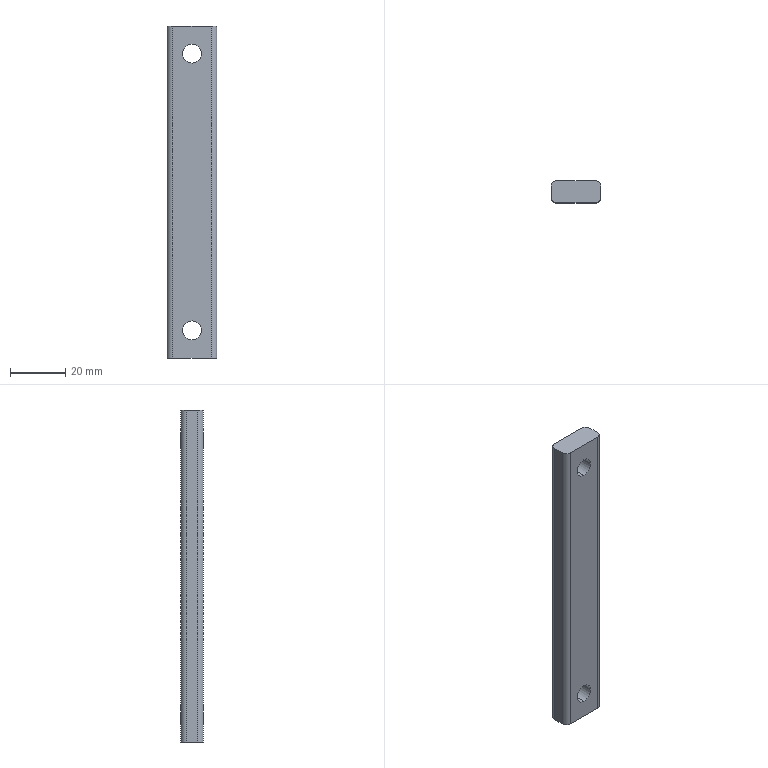Part | STEP file | Spring hanger hook | 1 solid | 14 faces | box 18 x 8 x 120 mm | volume 16287 mm3 | cylinder 8 | plane 6 | commonest cylinder face diameters 4 x4 6.8 x4
STEP:
#1=CARTESIAN_POINT('',(0.,0.,0.));
#2=DIRECTION('',(0.,0.,1.));
#3=DIRECTION('',(1.,0.,0.));
#4=AXIS2_PLACEMENT_3D('',#1,#2,#3);
#5=CARTESIAN_POINT('',(0.,4.,46.6));
#6=VERTEX_POINT('',#5);
#7=CARTESIAN_POINT('',(0.,-4.,46.6));
#8=VERTEX_POINT('',#7);
#9=CARTESIAN_POINT('',(0.,-4.,46.6));
#10=DIRECTION('',(0.,-1.,0.));
#11=VECTOR('',#10,1.);
#12=LINE('',#9,#11);
#13=CARTESIAN_POINT('',(0.,-4.,50.));
#14=DIRECTION('',(0.,-1.,0.));
#15=DIRECTION('',(0.,0.,-1.));
#16=AXIS2_PLACEMENT_3D('',#13,#14,#15);
#17=CYLINDRICAL_SURFACE('',#16,3.4);
#18=CARTESIAN_POINT('',(6.283,0.));
#19=DIRECTION('',(0.,1.));
#20=VECTOR('',#19,1.);
#21=LINE('',#18,#20);
#22=(GEOMETRIC_REPRESENTATION_CONTEXT(2)PARAMETRIC_REPRESENTATION_CONTEXT()REPRESENTATION_CONTEXT('',''));
#23=DEFINITIONAL_REPRESENTATION('',(#21),#22);
#24=PCURVE('',#17,#23);
#25=CARTESIAN_POINT('',(0.,-4.,50.));
#26=DIRECTION('',(0.,-1.,0.));
#27=DIRECTION('',(0.,0.,-1.));
#28=AXIS2_PLACEMENT_3D('',#25,#26,#27);
#29=CYLINDRICAL_SURFACE('',#28,3.4);
#30=CARTESIAN_POINT('',(0.,0.));
#31=DIRECTION('',(0.,1.));
#32=VECTOR('',#31,1.);
#33=LINE('',#30,#32);
#34=(GEOMETRIC_REPRESENTATION_CONTEXT(2)PARAMETRIC_REPRESENTATION_CONTEXT()REPRESENTATION_CONTEXT('',''));
#35=DEFINITIONAL_REPRESENTATION('',(#33),#34);
#36=PCURVE('',#29,#35);
#37=SURFACE_CURVE('',#12,(#24,#36),.PCURVE_S1.);
#38=EDGE_CURVE('',#6,#8,#37,.T.);
#39=ORIENTED_EDGE('',*,*,#38,.T.);
#40=CARTESIAN_POINT('',(0.,-4.,53.4));
#41=VERTEX_POINT('',#40);
#42=CARTESIAN_POINT('',(0.,-4.,50.));
#43=DIRECTION('',(0.,1.,0.));
#44=DIRECTION('',(0.,0.,-1.));
#45=AXIS2_PLACEMENT_3D('',#42,#43,#44);
#46=CIRCLE('',#45,3.4);
#47=CARTESIAN_POINT('',(6.283,0.));
#48=DIRECTION('',(-1.,0.));
#49=VECTOR('',#48,1.);
#50=LINE('',#47,#49);
#51=(GEOMETRIC_REPRESENTATION_CONTEXT(2)PARAMETRIC_REPRESENTATION_CONTEXT()REPRESENTATION_CONTEXT('',''));
#52=DEFINITIONAL_REPRESENTATION('',(#50),#51);
#53=PCURVE('',#17,#52);
#54=CARTESIAN_POINT('',(-9.,-4.,60.));
#55=DIRECTION('',(0.,1.,0.));
#56=DIRECTION('',(0.,0.,1.));
#57=AXIS2_PLACEMENT_3D('',#54,#55,#56);
#58=PLANE('',#57);
#59=CARTESIAN_POINT('',(-10.,9.));
#60=DIRECTION('',(-1.,0.));
#61=AXIS2_PLACEMENT_2D('',#59,#60);
#62=CIRCLE('',#61,3.4);
#63=(GEOMETRIC_REPRESENTATION_CONTEXT(2)PARAMETRIC_REPRESENTATION_CONTEXT()REPRESENTATION_CONTEXT('',''));
#64=DEFINITIONAL_REPRESENTATION('',(#62),#63);
#65=PCURVE('',#58,#64);
#66=SURFACE_CURVE('',#46,(#53,#65),.PCURVE_S1.);
#67=EDGE_CURVE('',#8,#41,#66,.T.);
#68=ORIENTED_EDGE('',*,*,#67,.T.);
#69=CARTESIAN_POINT('',(0.,4.,53.4));
#70=VERTEX_POINT('',#69);
#71=CARTESIAN_POINT('',(0.,-4.,53.4));
#72=DIRECTION('',(0.,-1.,0.));
#73=VECTOR('',#72,1.);
#74=LINE('',#71,#73);
#75=CARTESIAN_POINT('',(3.142,0.));
#76=DIRECTION('',(0.,1.));
#77=VECTOR('',#76,1.);
#78=LINE('',#75,#77);
#79=(GEOMETRIC_REPRESENTATION_CONTEXT(2)PARAMETRIC_REPRESENTATION_CONTEXT()REPRESENTATION_CONTEXT('',''));
#80=DEFINITIONAL_REPRESENTATION('',(#78),#79);
#81=PCURVE('',#17,#80);
#82=CARTESIAN_POINT('',(3.142,0.));
#83=DIRECTION('',(0.,1.));
#84=VECTOR('',#83,1.);
#85=LINE('',#82,#84);
#86=(GEOMETRIC_REPRESENTATION_CONTEXT(2)PARAMETRIC_REPRESENTATION_CONTEXT()REPRESENTATION_CONTEXT('',''));
#87=DEFINITIONAL_REPRESENTATION('',(#85),#86);
#88=PCURVE('',#29,#87);
#89=SURFACE_CURVE('',#74,(#81,#88),.PCURVE_S1.);
#90=EDGE_CURVE('',#70,#41,#89,.T.);
#91=ORIENTED_EDGE('',*,*,#90,.F.);
#92=CARTESIAN_POINT('',(0.,4.,50.));
#93=DIRECTION('',(0.,1.,0.));
#94=DIRECTION('',(0.,0.,-1.));
#95=AXIS2_PLACEMENT_3D('',#92,#93,#94);
#96=CIRCLE('',#95,3.4);
#97=CARTESIAN_POINT('',(6.283,-8.));
#98=DIRECTION('',(-1.,0.));
#99=VECTOR('',#98,1.);
#100=LINE('',#97,#99);
#101=(GEOMETRIC_REPRESENTATION_CONTEXT(2)PARAMETRIC_REPRESENTATION_CONTEXT()REPRESENTATION_CONTEXT('',''));
#102=DEFINITIONAL_REPRESENTATION('',(#100),#101);
#103=PCURVE('',#17,#102);
#104=CARTESIAN_POINT('',(-9.,4.,60.));
#105=DIRECTION('',(0.,-1.,0.));
#106=DIRECTION('',(0.,0.,-1.));
#107=AXIS2_PLACEMENT_3D('',#104,#105,#106);
#108=PLANE('',#107);
#109=CARTESIAN_POINT('',(13.4,9.));
#110=CARTESIAN_POINT('',(13.4,3.111));
#111=CARTESIAN_POINT('',(8.3,6.056));
#112=CARTESIAN_POINT('',(3.2,9.));
#113=CARTESIAN_POINT('',(8.3,11.944));
#114=CARTESIAN_POINT('',(13.4,14.889));
#115=CARTESIAN_POINT('',(13.4,9.));
#116=(BOUNDED_CURVE()B_SPLINE_CURVE(2,(#109,#110,#111,#112,#113,#114,#115),.UNSPECIFIED.,.T.,.F.)B_SPLINE_CURVE_WITH_KNOTS((1,2,2,2,2,1),(-2.094,0.,2.094,4.189,6.283,8.378),.UNSPECIFIED.)CURVE()GEOMETRIC_REPRESENTATION_ITEM()RATIONAL_B_SPLINE_CURVE((1.,0.5,1.,0.5,1.,0.5,1.))REPRESENTATION_ITEM(''));
#117=(GEOMETRIC_REPRESENTATION_CONTEXT(2)PARAMETRIC_REPRESENTATION_CONTEXT()REPRESENTATION_CONTEXT('',''));
#118=DEFINITIONAL_REPRESENTATION('',(#116),#117);
#119=PCURVE('',#108,#118);
#120=SURFACE_CURVE('',#96,(#103,#119),.PCURVE_S1.);
#121=EDGE_CURVE('',#6,#70,#120,.T.);
#122=ORIENTED_EDGE('',*,*,#121,.F.);
#123=EDGE_LOOP('',(#39,#68,#91,#122));
#124=FACE_BOUND('',#123,.F.);
#125=ADVANCED_FACE('',(#124),#17,.F.);
#126=CARTESIAN_POINT('',(0.,4.,-53.4));
#127=VERTEX_POINT('',#126);
#128=CARTESIAN_POINT('',(0.,-4.,-53.4));
#129=VERTEX_POINT('',#128);
#130=CARTESIAN_POINT('',(0.,-4.,-53.4));
#131=DIRECTION('',(0.,-1.,0.));
#132=VECTOR('',#131,1.);
#133=LINE('',#130,#132);
#134=CARTESIAN_POINT('',(0.,-4.,-50.));
#135=DIRECTION('',(0.,-1.,0.));
#136=DIRECTION('',(0.,0.,-1.));
#137=AXIS2_PLACEMENT_3D('',#134,#135,#136);
#138=CYLINDRICAL_SURFACE('',#137,3.4);
#139=CARTESIAN_POINT('',(6.283,0.));
#140=DIRECTION('',(0.,1.));
#141=VECTOR('',#140,1.);
#142=LINE('',#139,#141);
#143=(GEOMETRIC_REPRESENTATION_CONTEXT(2)PARAMETRIC_REPRESENTATION_CONTEXT()REPRESENTATION_CONTEXT('',''));
#144=DEFINITIONAL_REPRESENTATION('',(#142),#143);
#145=PCURVE('',#138,#144);
#146=CARTESIAN_POINT('',(0.,-4.,-50.));
#147=DIRECTION('',(0.,-1.,0.));
#148=DIRECTION('',(0.,0.,-1.));
#149=AXIS2_PLACEMENT_3D('',#146,#147,#148);
#150=CYLINDRICAL_SURFACE('',#149,3.4);
#151=CARTESIAN_POINT('',(0.,0.));
#152=DIRECTION('',(0.,1.));
#153=VECTOR('',#152,1.);
#154=LINE('',#151,#153);
#155=(GEOMETRIC_REPRESENTATION_CONTEXT(2)PARAMETRIC_REPRESENTATION_CONTEXT()REPRESENTATION_CONTEXT('',''));
#156=DEFINITIONAL_REPRESENTATION('',(#154),#155);
#157=PCURVE('',#150,#156);
#158=SURFACE_CURVE('',#133,(#145,#157),.PCURVE_S1.);
#159=EDGE_CURVE('',#127,#129,#158,.T.);
#160=ORIENTED_EDGE('',*,*,#159,.T.);
#161=CARTESIAN_POINT('',(0.,-4.,-46.6));
#162=VERTEX_POINT('',#161);
#163=CARTESIAN_POINT('',(0.,-4.,-50.));
#164=DIRECTION('',(0.,1.,0.));
#165=DIRECTION('',(0.,0.,-1.));
#166=AXIS2_PLACEMENT_3D('',#163,#164,#165);
#167=CIRCLE('',#166,3.4);
#168=CARTESIAN_POINT('',(6.283,0.));
#169=DIRECTION('',(-1.,0.));
#170=VECTOR('',#169,1.);
#171=LINE('',#168,#170);
#172=(GEOMETRIC_REPRESENTATION_CONTEXT(2)PARAMETRIC_REPRESENTATION_CONTEXT()REPRESENTATION_CONTEXT('',''));
#173=DEFINITIONAL_REPRESENTATION('',(#171),#172);
#174=PCURVE('',#138,#173);
#175=CARTESIAN_POINT('',(-110.,9.));
#176=DIRECTION('',(-1.,0.));
#177=AXIS2_PLACEMENT_2D('',#175,#176);
#178=CIRCLE('',#177,3.4);
#179=(GEOMETRIC_REPRESENTATION_CONTEXT(2)PARAMETRIC_REPRESENTATION_CONTEXT()REPRESENTATION_CONTEXT('',''));
#180=DEFINITIONAL_REPRESENTATION('',(#178),#179);
#181=PCURVE('',#58,#180);
#182=SURFACE_CURVE('',#167,(#174,#181),.PCURVE_S1.);
#183=EDGE_CURVE('',#129,#162,#182,.T.);
#184=ORIENTED_EDGE('',*,*,#183,.T.);
#185=CARTESIAN_POINT('',(0.,4.,-46.6));
#186=VERTEX_POINT('',#185);
#187=CARTESIAN_POINT('',(0.,-4.,-46.6));
#188=DIRECTION('',(0.,-1.,0.));
#189=VECTOR('',#188,1.);
#190=LINE('',#187,#189);
#191=CARTESIAN_POINT('',(3.142,0.));
#192=DIRECTION('',(0.,1.));
#193=VECTOR('',#192,1.);
#194=LINE('',#191,#193);
#195=(GEOMETRIC_REPRESENTATION_CONTEXT(2)PARAMETRIC_REPRESENTATION_CONTEXT()REPRESENTATION_CONTEXT('',''));
#196=DEFINITIONAL_REPRESENTATION('',(#194),#195);
#197=PCURVE('',#138,#196);
#198=CARTESIAN_POINT('',(3.142,0.));
#199=DIRECTION('',(0.,1.));
#200=VECTOR('',#199,1.);
#201=LINE('',#198,#200);
#202=(GEOMETRIC_REPRESENTATION_CONTEXT(2)PARAMETRIC_REPRESENTATION_CONTEXT()REPRESENTATION_CONTEXT('',''));
#203=DEFINITIONAL_REPRESENTATION('',(#201),#202);
#204=PCURVE('',#150,#203);
#205=SURFACE_CURVE('',#190,(#197,#204),.PCURVE_S1.);
#206=EDGE_CURVE('',#186,#162,#205,.T.);
#207=ORIENTED_EDGE('',*,*,#206,.F.);
#208=CARTESIAN_POINT('',(0.,4.,-50.));
#209=DIRECTION('',(0.,1.,0.));
#210=DIRECTION('',(0.,0.,-1.));
#211=AXIS2_PLACEMENT_3D('',#208,#209,#210);
#212=CIRCLE('',#211,3.4);
#213=CARTESIAN_POINT('',(6.283,-8.));
#214=DIRECTION('',(-1.,0.));
#215=VECTOR('',#214,1.);
#216=LINE('',#213,#215);
#217=(GEOMETRIC_REPRESENTATION_CONTEXT(2)PARAMETRIC_REPRESENTATION_CONTEXT()REPRESENTATION_CONTEXT('',''));
#218=DEFINITIONAL_REPRESENTATION('',(#216),#217);
#219=PCURVE('',#138,#218);
#220=CARTESIAN_POINT('',(113.4,9.));
#221=CARTESIAN_POINT('',(113.4,3.111));
#222=CARTESIAN_POINT('',(108.3,6.056));
#223=CARTESIAN_POINT('',(103.2,9.));
#224=CARTESIAN_POINT('',(108.3,11.944));
#225=CARTESIAN_POINT('',(113.4,14.889));
#226=CARTESIAN_POINT('',(113.4,9.));
#227=(BOUNDED_CURVE()B_SPLINE_CURVE(2,(#220,#221,#222,#223,#224,#225,#226),.UNSPECIFIED.,.T.,.F.)B_SPLINE_CURVE_WITH_KNOTS((1,2,2,2,2,1),(-2.094,0.,2.094,4.189,6.283,8.378),.UNSPECIFIED.)CURVE()GEOMETRIC_REPRESENTATION_ITEM()RATIONAL_B_SPLINE_CURVE((1.,0.5,1.,0.5,1.,0.5,1.))REPRESENTATION_ITEM(''));
#228=(GEOMETRIC_REPRESENTATION_CONTEXT(2)PARAMETRIC_REPRESENTATION_CONTEXT()REPRESENTATION_CONTEXT('',''));
#229=DEFINITIONAL_REPRESENTATION('',(#227),#228);
#230=PCURVE('',#108,#229);
#231=SURFACE_CURVE('',#212,(#219,#230),.PCURVE_S1.);
#232=EDGE_CURVE('',#127,#186,#231,.T.);
#233=ORIENTED_EDGE('',*,*,#232,.F.);
#234=EDGE_LOOP('',(#160,#184,#207,#233));
#235=FACE_BOUND('',#234,.F.);
#236=ADVANCED_FACE('',(#235),#138,.F.);
#237=CARTESIAN_POINT('',(-7.,4.,60.));
#238=VERTEX_POINT('',#237);
#239=CARTESIAN_POINT('',(-7.,4.,-60.));
#240=VERTEX_POINT('',#239);
#241=CARTESIAN_POINT('',(-7.,4.,60.));
#242=DIRECTION('',(0.,0.,-1.));
#243=VECTOR('',#242,1.);
#244=LINE('',#241,#243);
#245=CARTESIAN_POINT('',(0.,2.));
#246=DIRECTION('',(1.,0.));
#247=VECTOR('',#246,1.);
#248=LINE('',#245,#247);
#249=(GEOMETRIC_REPRESENTATION_CONTEXT(2)PARAMETRIC_REPRESENTATION_CONTEXT()REPRESENTATION_CONTEXT('',''));
#250=DEFINITIONAL_REPRESENTATION('',(#248),#249);
#251=PCURVE('',#108,#250);
#252=CARTESIAN_POINT('',(-7.,2.,60.));
#253=DIRECTION('',(0.,0.,-1.));
#254=DIRECTION('',(-1.,0.,0.));
#255=AXIS2_PLACEMENT_3D('',#252,#253,#254);
#256=CYLINDRICAL_SURFACE('',#255,2.);
#257=CARTESIAN_POINT('',(1.571,0.));
#258=DIRECTION('',(0.,1.));
#259=VECTOR('',#258,1.);
#260=LINE('',#257,#259);
#261=(GEOMETRIC_REPRESENTATION_CONTEXT(2)PARAMETRIC_REPRESENTATION_CONTEXT()REPRESENTATION_CONTEXT('',''));
#262=DEFINITIONAL_REPRESENTATION('',(#260),#261);
#263=PCURVE('',#256,#262);
#264=SURFACE_CURVE('',#244,(#251,#263),.PCURVE_S1.);
#265=EDGE_CURVE('',#238,#240,#264,.T.);
#266=ORIENTED_EDGE('',*,*,#265,.F.);
#267=CARTESIAN_POINT('',(7.,4.,60.));
#268=VERTEX_POINT('',#267);
#269=CARTESIAN_POINT('',(-9.,4.,60.));
#270=DIRECTION('',(-1.,0.,0.));
#271=VECTOR('',#270,1.);
#272=LINE('',#269,#271);
#273=CARTESIAN_POINT('',(0.,0.));
#274=DIRECTION('',(0.,-1.));
#275=VECTOR('',#274,1.);
#276=LINE('',#273,#275);
#277=(GEOMETRIC_REPRESENTATION_CONTEXT(2)PARAMETRIC_REPRESENTATION_CONTEXT()REPRESENTATION_CONTEXT('',''));
#278=DEFINITIONAL_REPRESENTATION('',(#276),#277);
#279=PCURVE('',#108,#278);
#280=CARTESIAN_POINT('',(9.,-4.,60.));
#281=DIRECTION('',(0.,0.,1.));
#282=DIRECTION('',(1.,0.,0.));
#283=AXIS2_PLACEMENT_3D('',#280,#281,#282);
#284=PLANE('',#283);
#285=CARTESIAN_POINT('',(-18.,8.));
#286=DIRECTION('',(-1.,0.));
#287=VECTOR('',#286,1.);
#288=LINE('',#285,#287);
#289=(GEOMETRIC_REPRESENTATION_CONTEXT(2)PARAMETRIC_REPRESENTATION_CONTEXT()REPRESENTATION_CONTEXT('',''));
#290=DEFINITIONAL_REPRESENTATION('',(#288),#289);
#291=PCURVE('',#284,#290);
#292=SURFACE_CURVE('',#272,(#279,#291),.PCURVE_S1.);
#293=EDGE_CURVE('',#268,#238,#292,.T.);
#294=ORIENTED_EDGE('',*,*,#293,.F.);
#295=CARTESIAN_POINT('',(7.,4.,-60.));
#296=VERTEX_POINT('',#295);
#297=CARTESIAN_POINT('',(7.,4.,60.));
#298=DIRECTION('',(0.,0.,1.));
#299=VECTOR('',#298,1.);
#300=LINE('',#297,#299);
#301=CARTESIAN_POINT('',(0.,16.));
#302=DIRECTION('',(-1.,0.));
#303=VECTOR('',#302,1.);
#304=LINE('',#301,#303);
#305=(GEOMETRIC_REPRESENTATION_CONTEXT(2)PARAMETRIC_REPRESENTATION_CONTEXT()REPRESENTATION_CONTEXT('',''));
#306=DEFINITIONAL_REPRESENTATION('',(#304),#305);
#307=PCURVE('',#108,#306);
#308=CARTESIAN_POINT('',(7.,2.,60.));
#309=DIRECTION('',(0.,0.,-1.));
#310=DIRECTION('',(-1.,0.,0.));
#311=AXIS2_PLACEMENT_3D('',#308,#309,#310);
#312=CYLINDRICAL_SURFACE('',#311,2.);
#313=CARTESIAN_POINT('',(1.571,0.));
#314=DIRECTION('',(0.,-1.));
#315=VECTOR('',#314,1.);
#316=LINE('',#313,#315);
#317=(GEOMETRIC_REPRESENTATION_CONTEXT(2)PARAMETRIC_REPRESENTATION_CONTEXT()REPRESENTATION_CONTEXT('',''));
#318=DEFINITIONAL_REPRESENTATION('',(#316),#317);
#319=PCURVE('',#312,#318);
#320=SURFACE_CURVE('',#300,(#307,#319),.PCURVE_S1.);
#321=EDGE_CURVE('',#296,#268,#320,.T.);
#322=ORIENTED_EDGE('',*,*,#321,.F.);
#323=CARTESIAN_POINT('',(-9.,4.,-60.));
#324=DIRECTION('',(1.,0.,0.));
#325=VECTOR('',#324,1.);
#326=LINE('',#323,#325);
#327=CARTESIAN_POINT('',(120.,0.));
#328=DIRECTION('',(0.,1.));
#329=VECTOR('',#328,1.);
#330=LINE('',#327,#329);
#331=(GEOMETRIC_REPRESENTATION_CONTEXT(2)PARAMETRIC_REPRESENTATION_CONTEXT()REPRESENTATION_CONTEXT('',''));
#332=DEFINITIONAL_REPRESENTATION('',(#330),#331);
#333=PCURVE('',#108,#332);
#334=CARTESIAN_POINT('',(9.,-4.,-60.));
#335=DIRECTION('',(0.,0.,1.));
#336=DIRECTION('',(1.,0.,0.));
#337=AXIS2_PLACEMENT_3D('',#334,#335,#336);
#338=PLANE('',#337);
#339=CARTESIAN_POINT('',(-18.,8.));
#340=DIRECTION('',(1.,0.));
#341=VECTOR('',#340,1.);
#342=LINE('',#339,#341);
#343=(GEOMETRIC_REPRESENTATION_CONTEXT(2)PARAMETRIC_REPRESENTATION_CONTEXT()REPRESENTATION_CONTEXT('',''));
#344=DEFINITIONAL_REPRESENTATION('',(#342),#343);
#345=PCURVE('',#338,#344);
#346=SURFACE_CURVE('',#326,(#333,#345),.PCURVE_S1.);
#347=EDGE_CURVE('',#240,#296,#346,.T.);
#348=ORIENTED_EDGE('',*,*,#347,.F.);
#349=EDGE_LOOP('',(#266,#294,#322,#348));
#350=FACE_BOUND('',#349,.T.);
#351=ORIENTED_EDGE('',*,*,#121,.F.);
#352=CARTESIAN_POINT('',(0.,4.,50.));
#353=DIRECTION('',(0.,1.,0.));
#354=DIRECTION('',(0.,0.,-1.));
#355=AXIS2_PLACEMENT_3D('',#352,#353,#354);
#356=CIRCLE('',#355,3.4);
#357=CARTESIAN_POINT('',(13.4,9.));
#358=CARTESIAN_POINT('',(13.4,3.111));
#359=CARTESIAN_POINT('',(8.3,6.056));
#360=CARTESIAN_POINT('',(3.2,9.));
#361=CARTESIAN_POINT('',(8.3,11.944));
#362=CARTESIAN_POINT('',(13.4,14.889));
#363=CARTESIAN_POINT('',(13.4,9.));
#364=(BOUNDED_CURVE()B_SPLINE_CURVE(2,(#357,#358,#359,#360,#361,#362,#363),.UNSPECIFIED.,.T.,.F.)B_SPLINE_CURVE_WITH_KNOTS((1,2,2,2,2,1),(-2.094,0.,2.094,4.189,6.283,8.378),.UNSPECIFIED.)CURVE()GEOMETRIC_REPRESENTATION_ITEM()RATIONAL_B_SPLINE_CURVE((1.,0.5,1.,0.5,1.,0.5,1.))REPRESENTATION_ITEM(''));
#365=(GEOMETRIC_REPRESENTATION_CONTEXT(2)PARAMETRIC_REPRESENTATION_CONTEXT()REPRESENTATION_CONTEXT('',''));
#366=DEFINITIONAL_REPRESENTATION('',(#364),#365);
#367=PCURVE('',#108,#366);
#368=CARTESIAN_POINT('',(6.283,-8.));
#369=DIRECTION('',(-1.,0.));
#370=VECTOR('',#369,1.);
#371=LINE('',#368,#370);
#372=(GEOMETRIC_REPRESENTATION_CONTEXT(2)PARAMETRIC_REPRESENTATION_CONTEXT()REPRESENTATION_CONTEXT('',''));
#373=DEFINITIONAL_REPRESENTATION('',(#371),#372);
#374=PCURVE('',#29,#373);
#375=SURFACE_CURVE('',#356,(#367,#374),.PCURVE_S1.);
#376=EDGE_CURVE('',#70,#6,#375,.T.);
#377=ORIENTED_EDGE('',*,*,#376,.F.);
#378=EDGE_LOOP('',(#351,#377));
#379=FACE_BOUND('',#378,.T.);
#380=ORIENTED_EDGE('',*,*,#232,.F.);
#381=CARTESIAN_POINT('',(0.,4.,-50.));
#382=DIRECTION('',(0.,1.,0.));
#383=DIRECTION('',(0.,0.,-1.));
#384=AXIS2_PLACEMENT_3D('',#381,#382,#383);
#385=CIRCLE('',#384,3.4);
#386=CARTESIAN_POINT('',(113.4,9.));
#387=CARTESIAN_POINT('',(113.4,3.111));
#388=CARTESIAN_POINT('',(108.3,6.056));
#389=CARTESIAN_POINT('',(103.2,9.));
#390=CARTESIAN_POINT('',(108.3,11.944));
#391=CARTESIAN_POINT('',(113.4,14.889));
#392=CARTESIAN_POINT('',(113.4,9.));
#393=(BOUNDED_CURVE()B_SPLINE_CURVE(2,(#386,#387,#388,#389,#390,#391,#392),.UNSPECIFIED.,.T.,.F.)B_SPLINE_CURVE_WITH_KNOTS((1,2,2,2,2,1),(-2.094,0.,2.094,4.189,6.283,8.378),.UNSPECIFIED.)CURVE()GEOMETRIC_REPRESENTATION_ITEM()RATIONAL_B_SPLINE_CURVE((1.,0.5,1.,0.5,1.,0.5,1.))REPRESENTATION_ITEM(''));
#394=(GEOMETRIC_REPRESENTATION_CONTEXT(2)PARAMETRIC_REPRESENTATION_CONTEXT()REPRESENTATION_CONTEXT('',''));
#395=DEFINITIONAL_REPRESENTATION('',(#393),#394);
#396=PCURVE('',#108,#395);
#397=CARTESIAN_POINT('',(6.283,-8.));
#398=DIRECTION('',(-1.,0.));
#399=VECTOR('',#398,1.);
#400=LINE('',#397,#399);
#401=(GEOMETRIC_REPRESENTATION_CONTEXT(2)PARAMETRIC_REPRESENTATION_CONTEXT()REPRESENTATION_CONTEXT('',''));
#402=DEFINITIONAL_REPRESENTATION('',(#400),#401);
#403=PCURVE('',#150,#402);
#404=SURFACE_CURVE('',#385,(#396,#403),.PCURVE_S1.);
#405=EDGE_CURVE('',#186,#127,#404,.T.);
#406=ORIENTED_EDGE('',*,*,#405,.F.);
#407=EDGE_LOOP('',(#380,#406));
#408=FACE_BOUND('',#407,.T.);
#409=ADVANCED_FACE('',(#350,#379,#408),#108,.F.);
#410=CARTESIAN_POINT('',(-9.,-2.,-60.));
#411=VERTEX_POINT('',#410);
#412=CARTESIAN_POINT('',(-7.,-4.,-60.));
#413=VERTEX_POINT('',#412);
#414=CARTESIAN_POINT('',(-7.,-2.,-60.));
#415=DIRECTION('',(0.,0.,1.));
#416=DIRECTION('',(-1.,0.,0.));
#417=AXIS2_PLACEMENT_3D('',#414,#415,#416);
#418=CIRCLE('',#417,2.);
#419=CARTESIAN_POINT('',(-16.,2.));
#420=DIRECTION('',(-1.,0.));
#421=AXIS2_PLACEMENT_2D('',#419,#420);
#422=CIRCLE('',#421,2.);
#423=(GEOMETRIC_REPRESENTATION_CONTEXT(2)PARAMETRIC_REPRESENTATION_CONTEXT()REPRESENTATION_CONTEXT('',''));
#424=DEFINITIONAL_REPRESENTATION('',(#422),#423);
#425=PCURVE('',#338,#424);
#426=CARTESIAN_POINT('',(-7.,-2.,60.));
#427=DIRECTION('',(0.,0.,-1.));
#428=DIRECTION('',(-1.,0.,0.));
#429=AXIS2_PLACEMENT_3D('',#426,#427,#428);
#430=CYLINDRICAL_SURFACE('',#429,2.);
#431=CARTESIAN_POINT('',(6.283,120.));
#432=DIRECTION('',(-1.,0.));
#433=VECTOR('',#432,1.);
#434=LINE('',#431,#433);
#435=(GEOMETRIC_REPRESENTATION_CONTEXT(2)PARAMETRIC_REPRESENTATION_CONTEXT()REPRESENTATION_CONTEXT('',''));
#436=DEFINITIONAL_REPRESENTATION('',(#434),#435);
#437=PCURVE('',#430,#436);
#438=SURFACE_CURVE('',#418,(#425,#437),.PCURVE_S1.);
#439=EDGE_CURVE('',#411,#413,#438,.T.);
#440=ORIENTED_EDGE('',*,*,#439,.F.);
#441=CARTESIAN_POINT('',(-9.,2.,-60.));
#442=VERTEX_POINT('',#441);
#443=CARTESIAN_POINT('',(-9.,-4.,-60.));
#444=DIRECTION('',(0.,-1.,0.));
#445=VECTOR('',#444,1.);
#446=LINE('',#443,#445);
#447=CARTESIAN_POINT('',(-18.,0.));
#448=DIRECTION('',(0.,-1.));
#449=VECTOR('',#448,1.);
#450=LINE('',#447,#449);
#451=(GEOMETRIC_REPRESENTATION_CONTEXT(2)PARAMETRIC_REPRESENTATION_CONTEXT()REPRESENTATION_CONTEXT('',''));
#452=DEFINITIONAL_REPRESENTATION('',(#450),#451);
#453=PCURVE('',#338,#452);
#454=CARTESIAN_POINT('',(-9.,4.,60.));
#455=DIRECTION('',(1.,0.,0.));
#456=DIRECTION('',(0.,1.,0.));
#457=AXIS2_PLACEMENT_3D('',#454,#455,#456);
#458=PLANE('',#457);
#459=CARTESIAN_POINT('',(-8.,-120.));
#460=DIRECTION('',(-1.,0.));
#461=VECTOR('',#460,1.);
#462=LINE('',#459,#461);
#463=(GEOMETRIC_REPRESENTATION_CONTEXT(2)PARAMETRIC_REPRESENTATION_CONTEXT()REPRESENTATION_CONTEXT('',''));
#464=DEFINITIONAL_REPRESENTATION('',(#462),#463);
#465=PCURVE('',#458,#464);
#466=SURFACE_CURVE('',#446,(#453,#465),.PCURVE_S1.);
#467=EDGE_CURVE('',#442,#411,#466,.T.);
#468=ORIENTED_EDGE('',*,*,#467,.F.);
#469=CARTESIAN_POINT('',(-7.,2.,-60.));
#470=DIRECTION('',(0.,0.,1.));
#471=DIRECTION('',(-1.,0.,0.));
#472=AXIS2_PLACEMENT_3D('',#469,#470,#471);
#473=CIRCLE('',#472,2.);
#474=CARTESIAN_POINT('',(-16.,6.));
#475=DIRECTION('',(-1.,0.));
#476=AXIS2_PLACEMENT_2D('',#474,#475);
#477=CIRCLE('',#476,2.);
#478=(GEOMETRIC_REPRESENTATION_CONTEXT(2)PARAMETRIC_REPRESENTATION_CONTEXT()REPRESENTATION_CONTEXT('',''));
#479=DEFINITIONAL_REPRESENTATION('',(#477),#478);
#480=PCURVE('',#338,#479);
#481=CARTESIAN_POINT('',(6.283,120.));
#482=DIRECTION('',(-1.,0.));
#483=VECTOR('',#482,1.);
#484=LINE('',#481,#483);
#485=(GEOMETRIC_REPRESENTATION_CONTEXT(2)PARAMETRIC_REPRESENTATION_CONTEXT()REPRESENTATION_CONTEXT('',''));
#486=DEFINITIONAL_REPRESENTATION('',(#484),#485);
#487=PCURVE('',#256,#486);
#488=SURFACE_CURVE('',#473,(#480,#487),.PCURVE_S1.);
#489=EDGE_CURVE('',#240,#442,#488,.T.);
#490=ORIENTED_EDGE('',*,*,#489,.F.);
#491=ORIENTED_EDGE('',*,*,#347,.T.);
#492=CARTESIAN_POINT('',(9.,2.,-60.));
#493=VERTEX_POINT('',#492);
#494=CARTESIAN_POINT('',(7.,2.,-60.));
#495=DIRECTION('',(0.,0.,1.));
#496=DIRECTION('',(-1.,0.,0.));
#497=AXIS2_PLACEMENT_3D('',#494,#495,#496);
#498=CIRCLE('',#497,2.);
#499=CARTESIAN_POINT('',(-2.,6.));
#500=DIRECTION('',(-1.,0.));
#501=AXIS2_PLACEMENT_2D('',#499,#500);
#502=CIRCLE('',#501,2.);
#503=(GEOMETRIC_REPRESENTATION_CONTEXT(2)PARAMETRIC_REPRESENTATION_CONTEXT()REPRESENTATION_CONTEXT('',''));
#504=DEFINITIONAL_REPRESENTATION('',(#502),#503);
#505=PCURVE('',#338,#504);
#506=CARTESIAN_POINT('',(6.283,120.));
#507=DIRECTION('',(-1.,0.));
#508=VECTOR('',#507,1.);
#509=LINE('',#506,#508);
#510=(GEOMETRIC_REPRESENTATION_CONTEXT(2)PARAMETRIC_REPRESENTATION_CONTEXT()REPRESENTATION_CONTEXT('',''));
#511=DEFINITIONAL_REPRESENTATION('',(#509),#510);
#512=PCURVE('',#312,#511);
#513=SURFACE_CURVE('',#498,(#505,#512),.PCURVE_S1.);
#514=EDGE_CURVE('',#493,#296,#513,.T.);
#515=ORIENTED_EDGE('',*,*,#514,.F.);
#516=CARTESIAN_POINT('',(9.,-2.,-60.));
#517=VERTEX_POINT('',#516);
#518=CARTESIAN_POINT('',(9.,-4.,-60.));
#519=DIRECTION('',(0.,1.,0.));
#520=VECTOR('',#519,1.);
#521=LINE('',#518,#520);
#522=CARTESIAN_POINT('',(0.,0.));
#523=DIRECTION('',(0.,1.));
#524=VECTOR('',#523,1.);
#525=LINE('',#522,#524);
#526=(GEOMETRIC_REPRESENTATION_CONTEXT(2)PARAMETRIC_REPRESENTATION_CONTEXT()REPRESENTATION_CONTEXT('',''));
#527=DEFINITIONAL_REPRESENTATION('',(#525),#526);
#528=PCURVE('',#338,#527);
#529=CARTESIAN_POINT('',(9.,4.,60.));
#530=DIRECTION('',(-1.,0.,0.));
#531=DIRECTION('',(0.,0.,1.));
#532=AXIS2_PLACEMENT_3D('',#529,#530,#531);
#533=PLANE('',#532);
#534=CARTESIAN_POINT('',(-120.,-8.));
#535=DIRECTION('',(0.,1.));
#536=VECTOR('',#535,1.);
#537=LINE('',#534,#536);
#538=(GEOMETRIC_REPRESENTATION_CONTEXT(2)PARAMETRIC_REPRESENTATION_CONTEXT()REPRESENTATION_CONTEXT('',''));
#539=DEFINITIONAL_REPRESENTATION('',(#537),#538);
#540=PCURVE('',#533,#539);
#541=SURFACE_CURVE('',#521,(#528,#540),.PCURVE_S1.);
#542=EDGE_CURVE('',#517,#493,#541,.T.);
#543=ORIENTED_EDGE('',*,*,#542,.F.);
#544=CARTESIAN_POINT('',(7.,-4.,-60.));
#545=VERTEX_POINT('',#544);
#546=CARTESIAN_POINT('',(7.,-2.,-60.));
#547=DIRECTION('',(0.,0.,1.));
#548=DIRECTION('',(-1.,0.,0.));
#549=AXIS2_PLACEMENT_3D('',#546,#547,#548);
#550=CIRCLE('',#549,2.);
#551=CARTESIAN_POINT('',(-2.,2.));
#552=DIRECTION('',(-1.,0.));
#553=AXIS2_PLACEMENT_2D('',#551,#552);
#554=CIRCLE('',#553,2.);
#555=(GEOMETRIC_REPRESENTATION_CONTEXT(2)PARAMETRIC_REPRESENTATION_CONTEXT()REPRESENTATION_CONTEXT('',''));
#556=DEFINITIONAL_REPRESENTATION('',(#554),#555);
#557=PCURVE('',#338,#556);
#558=CARTESIAN_POINT('',(7.,-2.,60.));
#559=DIRECTION('',(0.,0.,-1.));
#560=DIRECTION('',(-1.,0.,0.));
#561=AXIS2_PLACEMENT_3D('',#558,#559,#560);
#562=CYLINDRICAL_SURFACE('',#561,2.);
#563=CARTESIAN_POINT('',(6.283,120.));
#564=DIRECTION('',(-1.,0.));
#565=VECTOR('',#564,1.);
#566=LINE('',#563,#565);
#567=(GEOMETRIC_REPRESENTATION_CONTEXT(2)PARAMETRIC_REPRESENTATION_CONTEXT()REPRESENTATION_CONTEXT('',''));
#568=DEFINITIONAL_REPRESENTATION('',(#566),#567);
#569=PCURVE('',#562,#568);
#570=SURFACE_CURVE('',#550,(#557,#569),.PCURVE_S1.);
#571=EDGE_CURVE('',#545,#517,#570,.T.);
#572=ORIENTED_EDGE('',*,*,#571,.F.);
#573=CARTESIAN_POINT('',(9.,-4.,-60.));
#574=DIRECTION('',(1.,0.,0.));
#575=VECTOR('',#574,1.);
#576=LINE('',#573,#575);
#577=CARTESIAN_POINT('',(0.,0.));
#578=DIRECTION('',(1.,0.));
#579=VECTOR('',#578,1.);
#580=LINE('',#577,#579);
#581=(GEOMETRIC_REPRESENTATION_CONTEXT(2)PARAMETRIC_REPRESENTATION_CONTEXT()REPRESENTATION_CONTEXT('',''));
#582=DEFINITIONAL_REPRESENTATION('',(#580),#581);
#583=PCURVE('',#338,#582);
#584=CARTESIAN_POINT('',(-120.,18.));
#585=DIRECTION('',(0.,1.));
#586=VECTOR('',#585,1.);
#587=LINE('',#584,#586);
#588=(GEOMETRIC_REPRESENTATION_CONTEXT(2)PARAMETRIC_REPRESENTATION_CONTEXT()REPRESENTATION_CONTEXT('',''));
#589=DEFINITIONAL_REPRESENTATION('',(#587),#588);
#590=PCURVE('',#58,#589);
#591=SURFACE_CURVE('',#576,(#583,#590),.PCURVE_S1.);
#592=EDGE_CURVE('',#413,#545,#591,.T.);
#593=ORIENTED_EDGE('',*,*,#592,.F.);
#594=EDGE_LOOP('',(#440,#468,#490,#491,#515,#543,#572,#593));
#595=FACE_BOUND('',#594,.T.);
#596=ADVANCED_FACE('',(#595),#338,.F.);
#597=ORIENTED_EDGE('',*,*,#489,.T.);
#598=CARTESIAN_POINT('',(-9.,2.,60.));
#599=VERTEX_POINT('',#598);
#600=CARTESIAN_POINT('',(-9.,2.,60.));
#601=DIRECTION('',(0.,0.,1.));
#602=VECTOR('',#601,1.);
#603=LINE('',#600,#602);
#604=CARTESIAN_POINT('',(0.,0.));
#605=DIRECTION('',(0.,-1.));
#606=VECTOR('',#605,1.);
#607=LINE('',#604,#606);
#608=(GEOMETRIC_REPRESENTATION_CONTEXT(2)PARAMETRIC_REPRESENTATION_CONTEXT()REPRESENTATION_CONTEXT('',''));
#609=DEFINITIONAL_REPRESENTATION('',(#607),#608);
#610=PCURVE('',#256,#609);
#611=CARTESIAN_POINT('',(-2.,0.));
#612=DIRECTION('',(0.,1.));
#613=VECTOR('',#612,1.);
#614=LINE('',#611,#613);
#615=(GEOMETRIC_REPRESENTATION_CONTEXT(2)PARAMETRIC_REPRESENTATION_CONTEXT()REPRESENTATION_CONTEXT('',''));
#616=DEFINITIONAL_REPRESENTATION('',(#614),#615);
#617=PCURVE('',#458,#616);
#618=SURFACE_CURVE('',#603,(#610,#617),.PCURVE_S1.);
#619=EDGE_CURVE('',#442,#599,#618,.T.);
#620=ORIENTED_EDGE('',*,*,#619,.T.);
#621=CARTESIAN_POINT('',(-7.,2.,60.));
#622=DIRECTION('',(0.,0.,-1.));
#623=DIRECTION('',(-1.,0.,0.));
#624=AXIS2_PLACEMENT_3D('',#621,#622,#623);
#625=CIRCLE('',#624,2.);
#626=CARTESIAN_POINT('',(0.,0.));
#627=DIRECTION('',(1.,0.));
#628=VECTOR('',#627,1.);
#629=LINE('',#626,#628);
#630=(GEOMETRIC_REPRESENTATION_CONTEXT(2)PARAMETRIC_REPRESENTATION_CONTEXT()REPRESENTATION_CONTEXT('',''));
#631=DEFINITIONAL_REPRESENTATION('',(#629),#630);
#632=PCURVE('',#256,#631);
#633=CARTESIAN_POINT('',(-18.,6.));
#634=CARTESIAN_POINT('',(-18.,9.464));
#635=CARTESIAN_POINT('',(-15.,7.732));
#636=CARTESIAN_POINT('',(-12.,6.));
#637=CARTESIAN_POINT('',(-15.,4.268));
#638=CARTESIAN_POINT('',(-18.,2.536));
#639=CARTESIAN_POINT('',(-18.,6.));
#640=(BOUNDED_CURVE()B_SPLINE_CURVE(2,(#633,#634,#635,#636,#637,#638,#639),.UNSPECIFIED.,.T.,.F.)B_SPLINE_CURVE_WITH_KNOTS((1,2,2,2,2,1),(-2.094,0.,2.094,4.189,6.283,8.378),.UNSPECIFIED.)CURVE()GEOMETRIC_REPRESENTATION_ITEM()RATIONAL_B_SPLINE_CURVE((1.,0.5,1.,0.5,1.,0.5,1.))REPRESENTATION_ITEM(''));
#641=(GEOMETRIC_REPRESENTATION_CONTEXT(2)PARAMETRIC_REPRESENTATION_CONTEXT()REPRESENTATION_CONTEXT('',''));
#642=DEFINITIONAL_REPRESENTATION('',(#640),#641);
#643=PCURVE('',#284,#642);
#644=SURFACE_CURVE('',#625,(#632,#643),.PCURVE_S1.);
#645=EDGE_CURVE('',#599,#238,#644,.T.);
#646=ORIENTED_EDGE('',*,*,#645,.T.);
#647=ORIENTED_EDGE('',*,*,#265,.T.);
#648=EDGE_LOOP('',(#597,#620,#646,#647));
#649=FACE_BOUND('',#648,.T.);
#650=ADVANCED_FACE('',(#649),#256,.T.);
#651=ORIENTED_EDGE('',*,*,#293,.T.);
#652=ORIENTED_EDGE('',*,*,#645,.F.);
#653=CARTESIAN_POINT('',(-9.,-2.,60.));
#654=VERTEX_POINT('',#653);
#655=CARTESIAN_POINT('',(-9.,-4.,60.));
#656=DIRECTION('',(0.,-1.,0.));
#657=VECTOR('',#656,1.);
#658=LINE('',#655,#657);
#659=CARTESIAN_POINT('',(-18.,0.));
#660=DIRECTION('',(0.,-1.));
#661=VECTOR('',#660,1.);
#662=LINE('',#659,#661);
#663=(GEOMETRIC_REPRESENTATION_CONTEXT(2)PARAMETRIC_REPRESENTATION_CONTEXT()REPRESENTATION_CONTEXT('',''));
#664=DEFINITIONAL_REPRESENTATION('',(#662),#663);
#665=PCURVE('',#284,#664);
#666=CARTESIAN_POINT('',(-8.,0.));
#667=DIRECTION('',(-1.,0.));
#668=VECTOR('',#667,1.);
#669=LINE('',#666,#668);
#670=(GEOMETRIC_REPRESENTATION_CONTEXT(2)PARAMETRIC_REPRESENTATION_CONTEXT()REPRESENTATION_CONTEXT('',''));
#671=DEFINITIONAL_REPRESENTATION('',(#669),#670);
#672=PCURVE('',#458,#671);
#673=SURFACE_CURVE('',#658,(#665,#672),.PCURVE_S1.);
#674=EDGE_CURVE('',#599,#654,#673,.T.);
#675=ORIENTED_EDGE('',*,*,#674,.T.);
#676=CARTESIAN_POINT('',(-7.,-4.,60.));
#677=VERTEX_POINT('',#676);
#678=CARTESIAN_POINT('',(-7.,-2.,60.));
#679=DIRECTION('',(0.,0.,1.));
#680=DIRECTION('',(-1.,0.,0.));
#681=AXIS2_PLACEMENT_3D('',#678,#679,#680);
#682=CIRCLE('',#681,2.);
#683=CARTESIAN_POINT('',(-16.,2.));
#684=DIRECTION('',(-1.,0.));
#685=AXIS2_PLACEMENT_2D('',#683,#684);
#686=CIRCLE('',#685,2.);
#687=(GEOMETRIC_REPRESENTATION_CONTEXT(2)PARAMETRIC_REPRESENTATION_CONTEXT()REPRESENTATION_CONTEXT('',''));
#688=DEFINITIONAL_REPRESENTATION('',(#686),#687);
#689=PCURVE('',#284,#688);
#690=CARTESIAN_POINT('',(6.283,0.));
#691=DIRECTION('',(-1.,0.));
#692=VECTOR('',#691,1.);
#693=LINE('',#690,#692);
#694=(GEOMETRIC_REPRESENTATION_CONTEXT(2)PARAMETRIC_REPRESENTATION_CONTEXT()REPRESENTATION_CONTEXT('',''));
#695=DEFINITIONAL_REPRESENTATION('',(#693),#694);
#696=PCURVE('',#430,#695);
#697=SURFACE_CURVE('',#682,(#689,#696),.PCURVE_S1.);
#698=EDGE_CURVE('',#654,#677,#697,.T.);
#699=ORIENTED_EDGE('',*,*,#698,.T.);
#700=CARTESIAN_POINT('',(7.,-4.,60.));
#701=VERTEX_POINT('',#700);
#702=CARTESIAN_POINT('',(9.,-4.,60.));
#703=DIRECTION('',(1.,0.,0.));
#704=VECTOR('',#703,1.);
#705=LINE('',#702,#704);
#706=CARTESIAN_POINT('',(0.,0.));
#707=DIRECTION('',(1.,0.));
#708=VECTOR('',#707,1.);
#709=LINE('',#706,#708);
#710=(GEOMETRIC_REPRESENTATION_CONTEXT(2)PARAMETRIC_REPRESENTATION_CONTEXT()REPRESENTATION_CONTEXT('',''));
#711=DEFINITIONAL_REPRESENTATION('',(#709),#710);
#712=PCURVE('',#284,#711);
#713=CARTESIAN_POINT('',(0.,18.));
#714=DIRECTION('',(0.,1.));
#715=VECTOR('',#714,1.);
#716=LINE('',#713,#715);
#717=(GEOMETRIC_REPRESENTATION_CONTEXT(2)PARAMETRIC_REPRESENTATION_CONTEXT()REPRESENTATION_CONTEXT('',''));
#718=DEFINITIONAL_REPRESENTATION('',(#716),#717);
#719=PCURVE('',#58,#718);
#720=SURFACE_CURVE('',#705,(#712,#719),.PCURVE_S1.);
#721=EDGE_CURVE('',#677,#701,#720,.T.);
#722=ORIENTED_EDGE('',*,*,#721,.T.);
#723=CARTESIAN_POINT('',(9.,-2.,60.));
#724=VERTEX_POINT('',#723);
#725=CARTESIAN_POINT('',(7.,-2.,60.));
#726=DIRECTION('',(0.,0.,1.));
#727=DIRECTION('',(-1.,0.,0.));
#728=AXIS2_PLACEMENT_3D('',#725,#726,#727);
#729=CIRCLE('',#728,2.);
#730=CARTESIAN_POINT('',(-2.,2.));
#731=DIRECTION('',(-1.,0.));
#732=AXIS2_PLACEMENT_2D('',#730,#731);
#733=CIRCLE('',#732,2.);
#734=(GEOMETRIC_REPRESENTATION_CONTEXT(2)PARAMETRIC_REPRESENTATION_CONTEXT()REPRESENTATION_CONTEXT('',''));
#735=DEFINITIONAL_REPRESENTATION('',(#733),#734);
#736=PCURVE('',#284,#735);
#737=CARTESIAN_POINT('',(6.283,0.));
#738=DIRECTION('',(-1.,0.));
#739=VECTOR('',#738,1.);
#740=LINE('',#737,#739);
#741=(GEOMETRIC_REPRESENTATION_CONTEXT(2)PARAMETRIC_REPRESENTATION_CONTEXT()REPRESENTATION_CONTEXT('',''));
#742=DEFINITIONAL_REPRESENTATION('',(#740),#741);
#743=PCURVE('',#562,#742);
#744=SURFACE_CURVE('',#729,(#736,#743),.PCURVE_S1.);
#745=EDGE_CURVE('',#701,#724,#744,.T.);
#746=ORIENTED_EDGE('',*,*,#745,.T.);
#747=CARTESIAN_POINT('',(9.,2.,60.));
#748=VERTEX_POINT('',#747);
#749=CARTESIAN_POINT('',(9.,-4.,60.));
#750=DIRECTION('',(0.,1.,0.));
#751=VECTOR('',#750,1.);
#752=LINE('',#749,#751);
#753=CARTESIAN_POINT('',(0.,0.));
#754=DIRECTION('',(0.,1.));
#755=VECTOR('',#754,1.);
#756=LINE('',#753,#755);
#757=(GEOMETRIC_REPRESENTATION_CONTEXT(2)PARAMETRIC_REPRESENTATION_CONTEXT()REPRESENTATION_CONTEXT('',''));
#758=DEFINITIONAL_REPRESENTATION('',(#756),#757);
#759=PCURVE('',#284,#758);
#760=CARTESIAN_POINT('',(0.,-8.));
#761=DIRECTION('',(0.,1.));
#762=VECTOR('',#761,1.);
#763=LINE('',#760,#762);
#764=(GEOMETRIC_REPRESENTATION_CONTEXT(2)PARAMETRIC_REPRESENTATION_CONTEXT()REPRESENTATION_CONTEXT('',''));
#765=DEFINITIONAL_REPRESENTATION('',(#763),#764);
#766=PCURVE('',#533,#765);
#767=SURFACE_CURVE('',#752,(#759,#766),.PCURVE_S1.);
#768=EDGE_CURVE('',#724,#748,#767,.T.);
#769=ORIENTED_EDGE('',*,*,#768,.T.);
#770=CARTESIAN_POINT('',(7.,2.,60.));
#771=DIRECTION('',(0.,0.,1.));
#772=DIRECTION('',(-1.,0.,0.));
#773=AXIS2_PLACEMENT_3D('',#770,#771,#772);
#774=CIRCLE('',#773,2.);
#775=CARTESIAN_POINT('',(-2.,6.));
#776=DIRECTION('',(-1.,0.));
#777=AXIS2_PLACEMENT_2D('',#775,#776);
#778=CIRCLE('',#777,2.);
#779=(GEOMETRIC_REPRESENTATION_CONTEXT(2)PARAMETRIC_REPRESENTATION_CONTEXT()REPRESENTATION_CONTEXT('',''));
#780=DEFINITIONAL_REPRESENTATION('',(#778),#779);
#781=PCURVE('',#284,#780);
#782=CARTESIAN_POINT('',(6.283,0.));
#783=DIRECTION('',(-1.,0.));
#784=VECTOR('',#783,1.);
#785=LINE('',#782,#784);
#786=(GEOMETRIC_REPRESENTATION_CONTEXT(2)PARAMETRIC_REPRESENTATION_CONTEXT()REPRESENTATION_CONTEXT('',''));
#787=DEFINITIONAL_REPRESENTATION('',(#785),#786);
#788=PCURVE('',#312,#787);
#789=SURFACE_CURVE('',#774,(#781,#788),.PCURVE_S1.);
#790=EDGE_CURVE('',#748,#268,#789,.T.);
#791=ORIENTED_EDGE('',*,*,#790,.T.);
#792=EDGE_LOOP('',(#651,#652,#675,#699,#722,#746,#769,#791));
#793=FACE_BOUND('',#792,.T.);
#794=ADVANCED_FACE('',(#793),#284,.T.);
#795=ORIENTED_EDGE('',*,*,#514,.T.);
#796=ORIENTED_EDGE('',*,*,#321,.T.);
#797=ORIENTED_EDGE('',*,*,#790,.F.);
#798=CARTESIAN_POINT('',(9.,2.,60.));
#799=DIRECTION('',(0.,0.,-1.));
#800=VECTOR('',#799,1.);
#801=LINE('',#798,#800);
#802=CARTESIAN_POINT('',(3.142,0.));
#803=DIRECTION('',(0.,1.));
#804=VECTOR('',#803,1.);
#805=LINE('',#802,#804);
#806=(GEOMETRIC_REPRESENTATION_CONTEXT(2)PARAMETRIC_REPRESENTATION_CONTEXT()REPRESENTATION_CONTEXT('',''));
#807=DEFINITIONAL_REPRESENTATION('',(#805),#806);
#808=PCURVE('',#312,#807);
#809=CARTESIAN_POINT('',(0.,-2.));
#810=DIRECTION('',(-1.,0.));
#811=VECTOR('',#810,1.);
#812=LINE('',#809,#811);
#813=(GEOMETRIC_REPRESENTATION_CONTEXT(2)PARAMETRIC_REPRESENTATION_CONTEXT()REPRESENTATION_CONTEXT('',''));
#814=DEFINITIONAL_REPRESENTATION('',(#812),#813);
#815=PCURVE('',#533,#814);
#816=SURFACE_CURVE('',#801,(#808,#815),.PCURVE_S1.);
#817=EDGE_CURVE('',#748,#493,#816,.T.);
#818=ORIENTED_EDGE('',*,*,#817,.T.);
#819=EDGE_LOOP('',(#795,#796,#797,#818));
#820=FACE_BOUND('',#819,.T.);
#821=ADVANCED_FACE('',(#820),#312,.T.);
#822=CARTESIAN_POINT('',(0.,-4.,50.));
#823=DIRECTION('',(0.,1.,0.));
#824=DIRECTION('',(0.,0.,-1.));
#825=AXIS2_PLACEMENT_3D('',#822,#823,#824);
#826=CIRCLE('',#825,3.4);
#827=CARTESIAN_POINT('',(6.283,0.));
#828=DIRECTION('',(-1.,0.));
#829=VECTOR('',#828,1.);
#830=LINE('',#827,#829);
#831=(GEOMETRIC_REPRESENTATION_CONTEXT(2)PARAMETRIC_REPRESENTATION_CONTEXT()REPRESENTATION_CONTEXT('',''));
#832=DEFINITIONAL_REPRESENTATION('',(#830),#831);
#833=PCURVE('',#29,#832);
#834=CARTESIAN_POINT('',(-10.,9.));
#835=DIRECTION('',(-1.,0.));
#836=AXIS2_PLACEMENT_2D('',#834,#835);
#837=CIRCLE('',#836,3.4);
#838=(GEOMETRIC_REPRESENTATION_CONTEXT(2)PARAMETRIC_REPRESENTATION_CONTEXT()REPRESENTATION_CONTEXT('',''));
#839=DEFINITIONAL_REPRESENTATION('',(#837),#838);
#840=PCURVE('',#58,#839);
#841=SURFACE_CURVE('',#826,(#833,#840),.PCURVE_S1.);
#842=EDGE_CURVE('',#41,#8,#841,.T.);
#843=ORIENTED_EDGE('',*,*,#842,.T.);
#844=ORIENTED_EDGE('',*,*,#38,.F.);
#845=ORIENTED_EDGE('',*,*,#376,.F.);
#846=ORIENTED_EDGE('',*,*,#90,.T.);
#847=EDGE_LOOP('',(#843,#844,#845,#846));
#848=FACE_BOUND('',#847,.F.);
#849=ADVANCED_FACE('',(#848),#29,.F.);
#850=CARTESIAN_POINT('',(0.,-4.,-50.));
#851=DIRECTION('',(0.,1.,0.));
#852=DIRECTION('',(0.,0.,-1.));
#853=AXIS2_PLACEMENT_3D('',#850,#851,#852);
#854=CIRCLE('',#853,3.4);
#855=CARTESIAN_POINT('',(6.283,0.));
#856=DIRECTION('',(-1.,0.));
#857=VECTOR('',#856,1.);
#858=LINE('',#855,#857);
#859=(GEOMETRIC_REPRESENTATION_CONTEXT(2)PARAMETRIC_REPRESENTATION_CONTEXT()REPRESENTATION_CONTEXT('',''));
#860=DEFINITIONAL_REPRESENTATION('',(#858),#859);
#861=PCURVE('',#150,#860);
#862=CARTESIAN_POINT('',(-110.,9.));
#863=DIRECTION('',(-1.,0.));
#864=AXIS2_PLACEMENT_2D('',#862,#863);
#865=CIRCLE('',#864,3.4);
#866=(GEOMETRIC_REPRESENTATION_CONTEXT(2)PARAMETRIC_REPRESENTATION_CONTEXT()REPRESENTATION_CONTEXT('',''));
#867=DEFINITIONAL_REPRESENTATION('',(#865),#866);
#868=PCURVE('',#58,#867);
#869=SURFACE_CURVE('',#854,(#861,#868),.PCURVE_S1.);
#870=EDGE_CURVE('',#162,#129,#869,.T.);
#871=ORIENTED_EDGE('',*,*,#870,.T.);
#872=ORIENTED_EDGE('',*,*,#159,.F.);
#873=ORIENTED_EDGE('',*,*,#405,.F.);
#874=ORIENTED_EDGE('',*,*,#206,.T.);
#875=EDGE_LOOP('',(#871,#872,#873,#874));
#876=FACE_BOUND('',#875,.F.);
#877=ADVANCED_FACE('',(#876),#150,.F.);
#878=CARTESIAN_POINT('',(-7.,-4.,60.));
#879=DIRECTION('',(0.,0.,1.));
#880=VECTOR('',#879,1.);
#881=LINE('',#878,#880);
#882=CARTESIAN_POINT('',(0.,2.));
#883=DIRECTION('',(1.,0.));
#884=VECTOR('',#883,1.);
#885=LINE('',#882,#884);
#886=(GEOMETRIC_REPRESENTATION_CONTEXT(2)PARAMETRIC_REPRESENTATION_CONTEXT()REPRESENTATION_CONTEXT('',''));
#887=DEFINITIONAL_REPRESENTATION('',(#885),#886);
#888=PCURVE('',#58,#887);
#889=CARTESIAN_POINT('',(4.712,0.));
#890=DIRECTION('',(0.,-1.));
#891=VECTOR('',#890,1.);
#892=LINE('',#889,#891);
#893=(GEOMETRIC_REPRESENTATION_CONTEXT(2)PARAMETRIC_REPRESENTATION_CONTEXT()REPRESENTATION_CONTEXT('',''));
#894=DEFINITIONAL_REPRESENTATION('',(#892),#893);
#895=PCURVE('',#430,#894);
#896=SURFACE_CURVE('',#881,(#888,#895),.PCURVE_S1.);
#897=EDGE_CURVE('',#413,#677,#896,.T.);
#898=ORIENTED_EDGE('',*,*,#897,.F.);
#899=ORIENTED_EDGE('',*,*,#592,.T.);
#900=CARTESIAN_POINT('',(7.,-4.,60.));
#901=DIRECTION('',(0.,0.,-1.));
#902=VECTOR('',#901,1.);
#903=LINE('',#900,#902);
#904=CARTESIAN_POINT('',(0.,16.));
#905=DIRECTION('',(-1.,0.));
#906=VECTOR('',#905,1.);
#907=LINE('',#904,#906);
#908=(GEOMETRIC_REPRESENTATION_CONTEXT(2)PARAMETRIC_REPRESENTATION_CONTEXT()REPRESENTATION_CONTEXT('',''));
#909=DEFINITIONAL_REPRESENTATION('',(#907),#908);
#910=PCURVE('',#58,#909);
#911=CARTESIAN_POINT('',(4.712,0.));
#912=DIRECTION('',(0.,1.));
#913=VECTOR('',#912,1.);
#914=LINE('',#911,#913);
#915=(GEOMETRIC_REPRESENTATION_CONTEXT(2)PARAMETRIC_REPRESENTATION_CONTEXT()REPRESENTATION_CONTEXT('',''));
#916=DEFINITIONAL_REPRESENTATION('',(#914),#915);
#917=PCURVE('',#562,#916);
#918=SURFACE_CURVE('',#903,(#910,#917),.PCURVE_S1.);
#919=EDGE_CURVE('',#701,#545,#918,.T.);
#920=ORIENTED_EDGE('',*,*,#919,.F.);
#921=ORIENTED_EDGE('',*,*,#721,.F.);
#922=EDGE_LOOP('',(#898,#899,#920,#921));
#923=FACE_BOUND('',#922,.T.);
#924=ORIENTED_EDGE('',*,*,#67,.T.);
#925=ORIENTED_EDGE('',*,*,#842,.T.);
#926=EDGE_LOOP('',(#924,#925));
#927=FACE_BOUND('',#926,.T.);
#928=ORIENTED_EDGE('',*,*,#183,.T.);
#929=ORIENTED_EDGE('',*,*,#870,.T.);
#930=EDGE_LOOP('',(#928,#929));
#931=FACE_BOUND('',#930,.T.);
#932=ADVANCED_FACE('',(#923,#927,#931),#58,.F.);
#933=ORIENTED_EDGE('',*,*,#439,.T.);
#934=ORIENTED_EDGE('',*,*,#897,.T.);
#935=ORIENTED_EDGE('',*,*,#698,.F.);
#936=CARTESIAN_POINT('',(-9.,-2.,60.));
#937=DIRECTION('',(0.,0.,-1.));
#938=VECTOR('',#937,1.);
#939=LINE('',#936,#938);
#940=CARTESIAN_POINT('',(6.283,0.));
#941=DIRECTION('',(0.,1.));
#942=VECTOR('',#941,1.);
#943=LINE('',#940,#942);
#944=(GEOMETRIC_REPRESENTATION_CONTEXT(2)PARAMETRIC_REPRESENTATION_CONTEXT()REPRESENTATION_CONTEXT('',''));
#945=DEFINITIONAL_REPRESENTATION('',(#943),#944);
#946=PCURVE('',#430,#945);
#947=CARTESIAN_POINT('',(-6.,0.));
#948=DIRECTION('',(0.,-1.));
#949=VECTOR('',#948,1.);
#950=LINE('',#947,#949);
#951=(GEOMETRIC_REPRESENTATION_CONTEXT(2)PARAMETRIC_REPRESENTATION_CONTEXT()REPRESENTATION_CONTEXT('',''));
#952=DEFINITIONAL_REPRESENTATION('',(#950),#951);
#953=PCURVE('',#458,#952);
#954=SURFACE_CURVE('',#939,(#946,#953),.PCURVE_S1.);
#955=EDGE_CURVE('',#654,#411,#954,.T.);
#956=ORIENTED_EDGE('',*,*,#955,.T.);
#957=EDGE_LOOP('',(#933,#934,#935,#956));
#958=FACE_BOUND('',#957,.T.);
#959=ADVANCED_FACE('',(#958),#430,.T.);
#960=ORIENTED_EDGE('',*,*,#955,.F.);
#961=ORIENTED_EDGE('',*,*,#674,.F.);
#962=ORIENTED_EDGE('',*,*,#619,.F.);
#963=ORIENTED_EDGE('',*,*,#467,.T.);
#964=EDGE_LOOP('',(#960,#961,#962,#963));
#965=FACE_BOUND('',#964,.T.);
#966=ADVANCED_FACE('',(#965),#458,.F.);
#967=CARTESIAN_POINT('',(9.,-2.,60.));
#968=DIRECTION('',(0.,0.,1.));
#969=VECTOR('',#968,1.);
#970=LINE('',#967,#969);
#971=CARTESIAN_POINT('',(0.,-6.));
#972=DIRECTION('',(1.,0.));
#973=VECTOR('',#972,1.);
#974=LINE('',#971,#973);
#975=(GEOMETRIC_REPRESENTATION_CONTEXT(2)PARAMETRIC_REPRESENTATION_CONTEXT()REPRESENTATION_CONTEXT('',''));
#976=DEFINITIONAL_REPRESENTATION('',(#974),#975);
#977=PCURVE('',#533,#976);
#978=CARTESIAN_POINT('',(3.142,0.));
#979=DIRECTION('',(0.,-1.));
#980=VECTOR('',#979,1.);
#981=LINE('',#978,#980);
#982=(GEOMETRIC_REPRESENTATION_CONTEXT(2)PARAMETRIC_REPRESENTATION_CONTEXT()REPRESENTATION_CONTEXT('',''));
#983=DEFINITIONAL_REPRESENTATION('',(#981),#982);
#984=PCURVE('',#562,#983);
#985=SURFACE_CURVE('',#970,(#977,#984),.PCURVE_S1.);
#986=EDGE_CURVE('',#517,#724,#985,.T.);
#987=ORIENTED_EDGE('',*,*,#986,.F.);
#988=ORIENTED_EDGE('',*,*,#542,.T.);
#989=ORIENTED_EDGE('',*,*,#817,.F.);
#990=ORIENTED_EDGE('',*,*,#768,.F.);
#991=EDGE_LOOP('',(#987,#988,#989,#990));
#992=FACE_BOUND('',#991,.T.);
#993=ADVANCED_FACE('',(#992),#533,.F.);
#994=ORIENTED_EDGE('',*,*,#571,.T.);
#995=ORIENTED_EDGE('',*,*,#986,.T.);
#996=ORIENTED_EDGE('',*,*,#745,.F.);
#997=ORIENTED_EDGE('',*,*,#919,.T.);
#998=EDGE_LOOP('',(#994,#995,#996,#997));
#999=FACE_BOUND('',#998,.T.);
#1000=ADVANCED_FACE('',(#999),#562,.T.);
#1001=CLOSED_SHELL('',(#125,#236,#409,#596,#650,#794,#821,#849,#877,#932,#959,#966,#993,#1000));
#1002=MANIFOLD_SOLID_BREP('',#1001);
#1003=(LENGTH_UNIT()NAMED_UNIT(*)SI_UNIT(.MILLI.,.METRE.));
#1004=UNCERTAINTY_MEASURE_WITH_UNIT(LENGTH_MEASURE(0.0000001),#1003,'','');
#1005=(NAMED_UNIT(*)PLANE_ANGLE_UNIT()SI_UNIT($,.RADIAN.));
#1006=(NAMED_UNIT(*)SI_UNIT($,.STERADIAN.)SOLID_ANGLE_UNIT());
#1007=(GEOMETRIC_REPRESENTATION_CONTEXT(3)GLOBAL_UNCERTAINTY_ASSIGNED_CONTEXT((#1004))GLOBAL_UNIT_ASSIGNED_CONTEXT((#1003,#1005,#1006))REPRESENTATION_CONTEXT('',''));
#1008=ADVANCED_BREP_SHAPE_REPRESENTATION('',(#4,#1002),#1007);